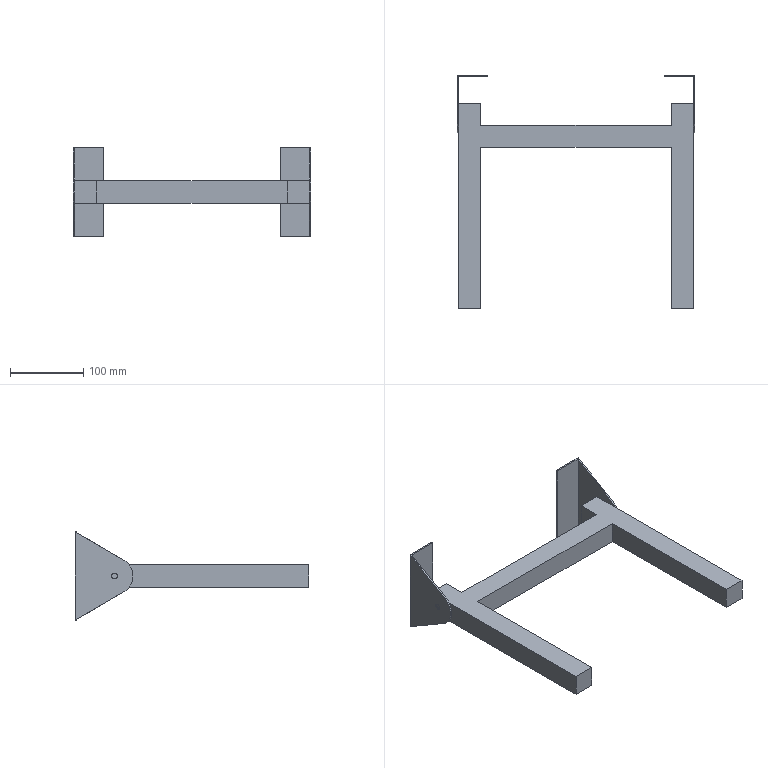Part | NX | 1 solid | 42 faces | box 324 x 318 x 120 mm | volume 780087 mm3 | plane 38 | cylinder 4 | commonest cylinder face diameters 8 x2 50 x2
STEP:
#1=CARTESIAN_POINT('',(-160.,140.,-15.));
#2=VERTEX_POINT('',#1);
#3=CARTESIAN_POINT('',(-160.,104.51,-15.));
#4=VERTEX_POINT('',#3);
#5=CARTESIAN_POINT('',(-160.,140.,-15.));
#6=DIRECTION('',(0.,-1.,0.));
#7=VECTOR('',#6,1.);
#8=LINE('',#5,#7);
#9=EDGE_CURVE('',#2,#4,#8,.T.);
#10=ORIENTED_EDGE('',*,*,#9,.F.);
#11=CARTESIAN_POINT('',(-130.,140.,-15.));
#12=VERTEX_POINT('',#11);
#13=CARTESIAN_POINT('',(-130.,140.,-15.));
#14=DIRECTION('',(-1.,0.,0.));
#15=VECTOR('',#14,1.);
#16=LINE('',#13,#15);
#17=EDGE_CURVE('',#12,#2,#16,.T.);
#18=ORIENTED_EDGE('',*,*,#17,.F.);
#19=CARTESIAN_POINT('',(-130.,110.,-15.));
#20=VERTEX_POINT('',#19);
#21=CARTESIAN_POINT('',(-130.,110.,-15.));
#22=DIRECTION('',(0.,1.,0.));
#23=VECTOR('',#22,1.);
#24=LINE('',#21,#23);
#25=EDGE_CURVE('',#20,#12,#24,.T.);
#26=ORIENTED_EDGE('',*,*,#25,.F.);
#27=CARTESIAN_POINT('',(130.,110.,-15.));
#28=VERTEX_POINT('',#27);
#29=CARTESIAN_POINT('',(130.,110.,-15.));
#30=DIRECTION('',(-1.,0.,0.));
#31=VECTOR('',#30,1.);
#32=LINE('',#29,#31);
#33=EDGE_CURVE('',#28,#20,#32,.T.);
#34=ORIENTED_EDGE('',*,*,#33,.F.);
#35=CARTESIAN_POINT('',(130.,140.,-15.));
#36=VERTEX_POINT('',#35);
#37=CARTESIAN_POINT('',(130.,140.,-15.));
#38=DIRECTION('',(0.,-1.,0.));
#39=VECTOR('',#38,1.);
#40=LINE('',#37,#39);
#41=EDGE_CURVE('',#36,#28,#40,.T.);
#42=ORIENTED_EDGE('',*,*,#41,.F.);
#43=CARTESIAN_POINT('',(160.,140.,-15.));
#44=VERTEX_POINT('',#43);
#45=CARTESIAN_POINT('',(160.,140.,-15.));
#46=DIRECTION('',(-1.,0.,0.));
#47=VECTOR('',#46,1.);
#48=LINE('',#45,#47);
#49=EDGE_CURVE('',#44,#36,#48,.T.);
#50=ORIENTED_EDGE('',*,*,#49,.F.);
#51=CARTESIAN_POINT('',(160.,104.51,-15.));
#52=VERTEX_POINT('',#51);
#53=CARTESIAN_POINT('',(160.,140.,-15.));
#54=DIRECTION('',(0.,-1.,0.));
#55=VECTOR('',#54,1.);
#56=LINE('',#53,#55);
#57=EDGE_CURVE('',#44,#52,#56,.T.);
#58=ORIENTED_EDGE('',*,*,#57,.T.);
#59=CARTESIAN_POINT('',(160.,-140.,-15.));
#60=VERTEX_POINT('',#59);
#61=CARTESIAN_POINT('',(160.,-140.,-15.));
#62=DIRECTION('',(0.,1.,0.));
#63=VECTOR('',#62,1.);
#64=LINE('',#61,#63);
#65=EDGE_CURVE('',#60,#52,#64,.T.);
#66=ORIENTED_EDGE('',*,*,#65,.F.);
#67=CARTESIAN_POINT('',(130.,-140.,-15.));
#68=VERTEX_POINT('',#67);
#69=CARTESIAN_POINT('',(130.,-140.,-15.));
#70=DIRECTION('',(1.,0.,0.));
#71=VECTOR('',#70,1.);
#72=LINE('',#69,#71);
#73=EDGE_CURVE('',#68,#60,#72,.T.);
#74=ORIENTED_EDGE('',*,*,#73,.F.);
#75=CARTESIAN_POINT('',(130.,80.,-15.));
#76=VERTEX_POINT('',#75);
#77=CARTESIAN_POINT('',(130.,80.,-15.));
#78=DIRECTION('',(0.,-1.,0.));
#79=VECTOR('',#78,1.);
#80=LINE('',#77,#79);
#81=EDGE_CURVE('',#76,#68,#80,.T.);
#82=ORIENTED_EDGE('',*,*,#81,.F.);
#83=CARTESIAN_POINT('',(-130.,80.,-15.));
#84=VERTEX_POINT('',#83);
#85=CARTESIAN_POINT('',(-130.,80.,-15.));
#86=DIRECTION('',(1.,0.,0.));
#87=VECTOR('',#86,1.);
#88=LINE('',#85,#87);
#89=EDGE_CURVE('',#84,#76,#88,.T.);
#90=ORIENTED_EDGE('',*,*,#89,.F.);
#91=CARTESIAN_POINT('',(-130.,-140.,-15.));
#92=VERTEX_POINT('',#91);
#93=CARTESIAN_POINT('',(-130.,-140.,-15.));
#94=DIRECTION('',(0.,1.,0.));
#95=VECTOR('',#94,1.);
#96=LINE('',#93,#95);
#97=EDGE_CURVE('',#92,#84,#96,.T.);
#98=ORIENTED_EDGE('',*,*,#97,.F.);
#99=CARTESIAN_POINT('',(-160.,-140.,-15.));
#100=VERTEX_POINT('',#99);
#101=CARTESIAN_POINT('',(-160.,-140.,-15.));
#102=DIRECTION('',(1.,0.,0.));
#103=VECTOR('',#102,1.);
#104=LINE('',#101,#103);
#105=EDGE_CURVE('',#100,#92,#104,.T.);
#106=ORIENTED_EDGE('',*,*,#105,.F.);
#107=CARTESIAN_POINT('',(-160.,104.51,-15.));
#108=DIRECTION('',(0.,-1.,0.));
#109=VECTOR('',#108,1.);
#110=LINE('',#107,#109);
#111=EDGE_CURVE('',#4,#100,#110,.T.);
#112=ORIENTED_EDGE('',*,*,#111,.F.);
#113=EDGE_LOOP('',(#10,#18,#26,#34,#42,#50,#58,#66,#74,#82,#90,#98,#106,#112));
#114=FACE_OUTER_BOUND('',#113,.T.);
#115=CARTESIAN_POINT('',(0.,0.,-15.));
#116=DIRECTION('',(0.,0.,1.));
#117=DIRECTION('',(1.,0.,0.));
#118=AXIS2_PLACEMENT_3D('',#115,#116,#117);
#119=PLANE('',#118);
#120=ADVANCED_FACE('',(#114),#119,.F.);
#121=CARTESIAN_POINT('',(-160.,140.,15.));
#122=VERTEX_POINT('',#121);
#123=CARTESIAN_POINT('',(-160.,104.51,15.));
#124=VERTEX_POINT('',#123);
#125=CARTESIAN_POINT('',(-160.,140.,15.));
#126=DIRECTION('',(0.,-1.,0.));
#127=VECTOR('',#126,1.);
#128=LINE('',#125,#127);
#129=EDGE_CURVE('',#122,#124,#128,.T.);
#130=ORIENTED_EDGE('',*,*,#129,.T.);
#131=CARTESIAN_POINT('',(-160.,-140.,15.));
#132=VERTEX_POINT('',#131);
#133=CARTESIAN_POINT('',(-160.,104.51,15.));
#134=DIRECTION('',(0.,-1.,0.));
#135=VECTOR('',#134,1.);
#136=LINE('',#133,#135);
#137=EDGE_CURVE('',#124,#132,#136,.T.);
#138=ORIENTED_EDGE('',*,*,#137,.T.);
#139=CARTESIAN_POINT('',(-130.,-140.,15.));
#140=VERTEX_POINT('',#139);
#141=CARTESIAN_POINT('',(-160.,-140.,15.));
#142=DIRECTION('',(1.,0.,0.));
#143=VECTOR('',#142,1.);
#144=LINE('',#141,#143);
#145=EDGE_CURVE('',#132,#140,#144,.T.);
#146=ORIENTED_EDGE('',*,*,#145,.T.);
#147=CARTESIAN_POINT('',(-130.,80.,15.));
#148=VERTEX_POINT('',#147);
#149=CARTESIAN_POINT('',(-130.,-140.,15.));
#150=DIRECTION('',(0.,1.,0.));
#151=VECTOR('',#150,1.);
#152=LINE('',#149,#151);
#153=EDGE_CURVE('',#140,#148,#152,.T.);
#154=ORIENTED_EDGE('',*,*,#153,.T.);
#155=CARTESIAN_POINT('',(130.,80.,15.));
#156=VERTEX_POINT('',#155);
#157=CARTESIAN_POINT('',(-130.,80.,15.));
#158=DIRECTION('',(1.,0.,0.));
#159=VECTOR('',#158,1.);
#160=LINE('',#157,#159);
#161=EDGE_CURVE('',#148,#156,#160,.T.);
#162=ORIENTED_EDGE('',*,*,#161,.T.);
#163=CARTESIAN_POINT('',(130.,-140.,15.));
#164=VERTEX_POINT('',#163);
#165=CARTESIAN_POINT('',(130.,80.,15.));
#166=DIRECTION('',(0.,-1.,0.));
#167=VECTOR('',#166,1.);
#168=LINE('',#165,#167);
#169=EDGE_CURVE('',#156,#164,#168,.T.);
#170=ORIENTED_EDGE('',*,*,#169,.T.);
#171=CARTESIAN_POINT('',(160.,-140.,15.));
#172=VERTEX_POINT('',#171);
#173=CARTESIAN_POINT('',(130.,-140.,15.));
#174=DIRECTION('',(1.,0.,0.));
#175=VECTOR('',#174,1.);
#176=LINE('',#173,#175);
#177=EDGE_CURVE('',#164,#172,#176,.T.);
#178=ORIENTED_EDGE('',*,*,#177,.T.);
#179=CARTESIAN_POINT('',(160.,104.51,15.));
#180=VERTEX_POINT('',#179);
#181=CARTESIAN_POINT('',(160.,-140.,15.));
#182=DIRECTION('',(0.,1.,0.));
#183=VECTOR('',#182,1.);
#184=LINE('',#181,#183);
#185=EDGE_CURVE('',#172,#180,#184,.T.);
#186=ORIENTED_EDGE('',*,*,#185,.T.);
#187=CARTESIAN_POINT('',(160.,140.,15.));
#188=VERTEX_POINT('',#187);
#189=CARTESIAN_POINT('',(160.,140.,15.));
#190=DIRECTION('',(0.,-1.,0.));
#191=VECTOR('',#190,1.);
#192=LINE('',#189,#191);
#193=EDGE_CURVE('',#188,#180,#192,.T.);
#194=ORIENTED_EDGE('',*,*,#193,.F.);
#195=CARTESIAN_POINT('',(130.,140.,15.));
#196=VERTEX_POINT('',#195);
#197=CARTESIAN_POINT('',(160.,140.,15.));
#198=DIRECTION('',(-1.,0.,0.));
#199=VECTOR('',#198,1.);
#200=LINE('',#197,#199);
#201=EDGE_CURVE('',#188,#196,#200,.T.);
#202=ORIENTED_EDGE('',*,*,#201,.T.);
#203=CARTESIAN_POINT('',(130.,110.,15.));
#204=VERTEX_POINT('',#203);
#205=CARTESIAN_POINT('',(130.,140.,15.));
#206=DIRECTION('',(0.,-1.,0.));
#207=VECTOR('',#206,1.);
#208=LINE('',#205,#207);
#209=EDGE_CURVE('',#196,#204,#208,.T.);
#210=ORIENTED_EDGE('',*,*,#209,.T.);
#211=CARTESIAN_POINT('',(-130.,110.,15.));
#212=VERTEX_POINT('',#211);
#213=CARTESIAN_POINT('',(130.,110.,15.));
#214=DIRECTION('',(-1.,0.,0.));
#215=VECTOR('',#214,1.);
#216=LINE('',#213,#215);
#217=EDGE_CURVE('',#204,#212,#216,.T.);
#218=ORIENTED_EDGE('',*,*,#217,.T.);
#219=CARTESIAN_POINT('',(-130.,140.,15.));
#220=VERTEX_POINT('',#219);
#221=CARTESIAN_POINT('',(-130.,110.,15.));
#222=DIRECTION('',(0.,1.,0.));
#223=VECTOR('',#222,1.);
#224=LINE('',#221,#223);
#225=EDGE_CURVE('',#212,#220,#224,.T.);
#226=ORIENTED_EDGE('',*,*,#225,.T.);
#227=CARTESIAN_POINT('',(-130.,140.,15.));
#228=DIRECTION('',(-1.,0.,0.));
#229=VECTOR('',#228,1.);
#230=LINE('',#227,#229);
#231=EDGE_CURVE('',#220,#122,#230,.T.);
#232=ORIENTED_EDGE('',*,*,#231,.T.);
#233=EDGE_LOOP('',(#130,#138,#146,#154,#162,#170,#178,#186,#194,#202,#210,#218,#226,#232));
#234=FACE_OUTER_BOUND('',#233,.T.);
#235=CARTESIAN_POINT('',(0.,0.,15.));
#236=DIRECTION('',(0.,0.,1.));
#237=DIRECTION('',(1.,0.,0.));
#238=AXIS2_PLACEMENT_3D('',#235,#236,#237);
#239=PLANE('',#238);
#240=ADVANCED_FACE('',(#234),#239,.T.);
#241=CARTESIAN_POINT('',(130.,80.,-15.));
#242=DIRECTION('',(0.,0.,1.));
#243=VECTOR('',#242,1.);
#244=LINE('',#241,#243);
#245=EDGE_CURVE('',#76,#156,#244,.T.);
#246=ORIENTED_EDGE('',*,*,#245,.F.);
#247=ORIENTED_EDGE('',*,*,#81,.T.);
#248=CARTESIAN_POINT('',(130.,-140.,-15.));
#249=DIRECTION('',(0.,0.,1.));
#250=VECTOR('',#249,1.);
#251=LINE('',#248,#250);
#252=EDGE_CURVE('',#68,#164,#251,.T.);
#253=ORIENTED_EDGE('',*,*,#252,.T.);
#254=ORIENTED_EDGE('',*,*,#169,.F.);
#255=EDGE_LOOP('',(#246,#247,#253,#254));
#256=FACE_OUTER_BOUND('',#255,.T.);
#257=CARTESIAN_POINT('',(130.,140.,-15.));
#258=DIRECTION('',(-1.,0.,0.));
#259=DIRECTION('',(0.,0.,1.));
#260=AXIS2_PLACEMENT_3D('',#257,#258,#259);
#261=PLANE('',#260);
#262=ADVANCED_FACE('',(#256),#261,.T.);
#263=CARTESIAN_POINT('',(130.,110.,-15.));
#264=DIRECTION('',(0.,0.,1.));
#265=VECTOR('',#264,1.);
#266=LINE('',#263,#265);
#267=EDGE_CURVE('',#28,#204,#266,.T.);
#268=ORIENTED_EDGE('',*,*,#267,.T.);
#269=ORIENTED_EDGE('',*,*,#209,.F.);
#270=CARTESIAN_POINT('',(130.,140.,-15.));
#271=DIRECTION('',(0.,0.,1.));
#272=VECTOR('',#271,1.);
#273=LINE('',#270,#272);
#274=EDGE_CURVE('',#36,#196,#273,.T.);
#275=ORIENTED_EDGE('',*,*,#274,.F.);
#276=ORIENTED_EDGE('',*,*,#41,.T.);
#277=EDGE_LOOP('',(#268,#269,#275,#276));
#278=FACE_OUTER_BOUND('',#277,.T.);
#279=CARTESIAN_POINT('',(130.,140.,-15.));
#280=DIRECTION('',(-1.,0.,0.));
#281=DIRECTION('',(0.,0.,1.));
#282=AXIS2_PLACEMENT_3D('',#279,#280,#281);
#283=PLANE('',#282);
#284=ADVANCED_FACE('',(#278),#283,.T.);
#285=ORIENTED_EDGE('',*,*,#73,.T.);
#286=CARTESIAN_POINT('',(160.,-140.,-15.));
#287=DIRECTION('',(0.,0.,1.));
#288=VECTOR('',#287,1.);
#289=LINE('',#286,#288);
#290=EDGE_CURVE('',#60,#172,#289,.T.);
#291=ORIENTED_EDGE('',*,*,#290,.T.);
#292=ORIENTED_EDGE('',*,*,#177,.F.);
#293=ORIENTED_EDGE('',*,*,#252,.F.);
#294=EDGE_LOOP('',(#285,#291,#292,#293));
#295=FACE_OUTER_BOUND('',#294,.T.);
#296=CARTESIAN_POINT('',(130.,-140.,-15.));
#297=DIRECTION('',(0.,-1.,0.));
#298=DIRECTION('',(0.,0.,-1.));
#299=AXIS2_PLACEMENT_3D('',#296,#297,#298);
#300=PLANE('',#299);
#301=ADVANCED_FACE('',(#295),#300,.T.);
#302=ORIENTED_EDGE('',*,*,#65,.T.);
#303=CARTESIAN_POINT('',(160.,124.51,0.));
#304=DIRECTION('',(1.,0.,0.));
#305=DIRECTION('',(0.,-0.8,0.6));
#306=AXIS2_PLACEMENT_3D('',#303,#304,#305);
#307=CIRCLE('',#306,25.);
#308=EDGE_CURVE('',#180,#52,#307,.T.);
#309=ORIENTED_EDGE('',*,*,#308,.F.);
#310=ORIENTED_EDGE('',*,*,#185,.F.);
#311=ORIENTED_EDGE('',*,*,#290,.F.);
#312=EDGE_LOOP('',(#302,#309,#310,#311));
#313=FACE_OUTER_BOUND('',#312,.T.);
#314=CARTESIAN_POINT('',(160.,-140.,-15.));
#315=DIRECTION('',(1.,0.,0.));
#316=DIRECTION('',(0.,0.,-1.));
#317=AXIS2_PLACEMENT_3D('',#314,#315,#316);
#318=PLANE('',#317);
#319=ADVANCED_FACE('',(#313),#318,.T.);
#320=CARTESIAN_POINT('',(160.,120.51,0.));
#321=VERTEX_POINT('',#320);
#322=CARTESIAN_POINT('',(160.,124.51,0.));
#323=DIRECTION('',(1.,0.,0.));
#324=DIRECTION('',(0.,1.,0.));
#325=AXIS2_PLACEMENT_3D('',#322,#323,#324);
#326=CIRCLE('',#325,4.);
#327=EDGE_CURVE('',#321,#321,#326,.T.);
#328=ORIENTED_EDGE('',*,*,#327,.T.);
#329=EDGE_LOOP('',(#328));
#330=FACE_OUTER_BOUND('',#329,.T.);
#331=CARTESIAN_POINT('',(160.,-140.,-15.));
#332=DIRECTION('',(1.,0.,0.));
#333=DIRECTION('',(0.,0.,-1.));
#334=AXIS2_PLACEMENT_3D('',#331,#332,#333);
#335=PLANE('',#334);
#336=ADVANCED_FACE('',(#330),#335,.T.);
#337=ORIENTED_EDGE('',*,*,#49,.T.);
#338=ORIENTED_EDGE('',*,*,#274,.T.);
#339=ORIENTED_EDGE('',*,*,#201,.F.);
#340=CARTESIAN_POINT('',(160.,140.,-15.));
#341=DIRECTION('',(0.,0.,1.));
#342=VECTOR('',#341,1.);
#343=LINE('',#340,#342);
#344=EDGE_CURVE('',#44,#188,#343,.T.);
#345=ORIENTED_EDGE('',*,*,#344,.F.);
#346=EDGE_LOOP('',(#337,#338,#339,#345));
#347=FACE_OUTER_BOUND('',#346,.T.);
#348=CARTESIAN_POINT('',(160.,140.,-15.));
#349=DIRECTION('',(0.,1.,0.));
#350=DIRECTION('',(0.,0.,1.));
#351=AXIS2_PLACEMENT_3D('',#348,#349,#350);
#352=PLANE('',#351);
#353=ADVANCED_FACE('',(#347),#352,.T.);
#354=CARTESIAN_POINT('',(-160.,140.,-15.));
#355=DIRECTION('',(0.,0.,1.));
#356=VECTOR('',#355,1.);
#357=LINE('',#354,#356);
#358=EDGE_CURVE('',#2,#122,#357,.T.);
#359=ORIENTED_EDGE('',*,*,#358,.T.);
#360=ORIENTED_EDGE('',*,*,#231,.F.);
#361=CARTESIAN_POINT('',(-130.,140.,-15.));
#362=DIRECTION('',(0.,0.,1.));
#363=VECTOR('',#362,1.);
#364=LINE('',#361,#363);
#365=EDGE_CURVE('',#12,#220,#364,.T.);
#366=ORIENTED_EDGE('',*,*,#365,.F.);
#367=ORIENTED_EDGE('',*,*,#17,.T.);
#368=EDGE_LOOP('',(#359,#360,#366,#367));
#369=FACE_OUTER_BOUND('',#368,.T.);
#370=CARTESIAN_POINT('',(-130.,140.,-15.));
#371=DIRECTION('',(0.,1.,0.));
#372=DIRECTION('',(0.,0.,1.));
#373=AXIS2_PLACEMENT_3D('',#370,#371,#372);
#374=PLANE('',#373);
#375=ADVANCED_FACE('',(#369),#374,.T.);
#376=CARTESIAN_POINT('',(-160.,128.51,0.));
#377=VERTEX_POINT('',#376);
#378=CARTESIAN_POINT('',(-160.,124.51,0.));
#379=DIRECTION('',(1.,0.,0.));
#380=DIRECTION('',(0.,1.,0.));
#381=AXIS2_PLACEMENT_3D('',#378,#379,#380);
#382=CIRCLE('',#381,4.);
#383=EDGE_CURVE('',#377,#377,#382,.T.);
#384=ORIENTED_EDGE('',*,*,#383,.F.);
#385=EDGE_LOOP('',(#384));
#386=FACE_OUTER_BOUND('',#385,.T.);
#387=CARTESIAN_POINT('',(-160.,140.,-15.));
#388=DIRECTION('',(-1.,0.,0.));
#389=DIRECTION('',(0.,0.,1.));
#390=AXIS2_PLACEMENT_3D('',#387,#388,#389);
#391=PLANE('',#390);
#392=ADVANCED_FACE('',(#386),#391,.T.);
#393=CARTESIAN_POINT('',(-160.,124.51,0.));
#394=DIRECTION('',(1.,0.,0.));
#395=DIRECTION('',(0.,-0.8,0.6));
#396=AXIS2_PLACEMENT_3D('',#393,#394,#395);
#397=CIRCLE('',#396,25.);
#398=EDGE_CURVE('',#124,#4,#397,.T.);
#399=ORIENTED_EDGE('',*,*,#398,.T.);
#400=ORIENTED_EDGE('',*,*,#111,.T.);
#401=CARTESIAN_POINT('',(-160.,-140.,-15.));
#402=DIRECTION('',(0.,0.,1.));
#403=VECTOR('',#402,1.);
#404=LINE('',#401,#403);
#405=EDGE_CURVE('',#100,#132,#404,.T.);
#406=ORIENTED_EDGE('',*,*,#405,.T.);
#407=ORIENTED_EDGE('',*,*,#137,.F.);
#408=EDGE_LOOP('',(#399,#400,#406,#407));
#409=FACE_OUTER_BOUND('',#408,.T.);
#410=CARTESIAN_POINT('',(-160.,140.,-15.));
#411=DIRECTION('',(-1.,0.,0.));
#412=DIRECTION('',(0.,0.,1.));
#413=AXIS2_PLACEMENT_3D('',#410,#411,#412);
#414=PLANE('',#413);
#415=ADVANCED_FACE('',(#409),#414,.T.);
#416=ORIENTED_EDGE('',*,*,#105,.T.);
#417=CARTESIAN_POINT('',(-130.,-140.,-15.));
#418=DIRECTION('',(0.,0.,1.));
#419=VECTOR('',#418,1.);
#420=LINE('',#417,#419);
#421=EDGE_CURVE('',#92,#140,#420,.T.);
#422=ORIENTED_EDGE('',*,*,#421,.T.);
#423=ORIENTED_EDGE('',*,*,#145,.F.);
#424=ORIENTED_EDGE('',*,*,#405,.F.);
#425=EDGE_LOOP('',(#416,#422,#423,#424));
#426=FACE_OUTER_BOUND('',#425,.T.);
#427=CARTESIAN_POINT('',(-160.,-140.,-15.));
#428=DIRECTION('',(0.,-1.,0.));
#429=DIRECTION('',(0.,0.,-1.));
#430=AXIS2_PLACEMENT_3D('',#427,#428,#429);
#431=PLANE('',#430);
#432=ADVANCED_FACE('',(#426),#431,.T.);
#433=CARTESIAN_POINT('',(-130.,80.,-15.));
#434=DIRECTION('',(0.,0.,1.));
#435=VECTOR('',#434,1.);
#436=LINE('',#433,#435);
#437=EDGE_CURVE('',#84,#148,#436,.T.);
#438=ORIENTED_EDGE('',*,*,#437,.T.);
#439=ORIENTED_EDGE('',*,*,#153,.F.);
#440=ORIENTED_EDGE('',*,*,#421,.F.);
#441=ORIENTED_EDGE('',*,*,#97,.T.);
#442=EDGE_LOOP('',(#438,#439,#440,#441));
#443=FACE_OUTER_BOUND('',#442,.T.);
#444=CARTESIAN_POINT('',(-130.,-140.,-15.));
#445=DIRECTION('',(1.,0.,0.));
#446=DIRECTION('',(0.,0.,-1.));
#447=AXIS2_PLACEMENT_3D('',#444,#445,#446);
#448=PLANE('',#447);
#449=ADVANCED_FACE('',(#443),#448,.T.);
#450=CARTESIAN_POINT('',(-130.,110.,-15.));
#451=DIRECTION('',(0.,0.,1.));
#452=VECTOR('',#451,1.);
#453=LINE('',#450,#452);
#454=EDGE_CURVE('',#20,#212,#453,.T.);
#455=ORIENTED_EDGE('',*,*,#454,.F.);
#456=ORIENTED_EDGE('',*,*,#25,.T.);
#457=ORIENTED_EDGE('',*,*,#365,.T.);
#458=ORIENTED_EDGE('',*,*,#225,.F.);
#459=EDGE_LOOP('',(#455,#456,#457,#458));
#460=FACE_OUTER_BOUND('',#459,.T.);
#461=CARTESIAN_POINT('',(-130.,-140.,-15.));
#462=DIRECTION('',(1.,0.,0.));
#463=DIRECTION('',(0.,0.,-1.));
#464=AXIS2_PLACEMENT_3D('',#461,#462,#463);
#465=PLANE('',#464);
#466=ADVANCED_FACE('',(#460),#465,.T.);
#467=ORIENTED_EDGE('',*,*,#245,.T.);
#468=ORIENTED_EDGE('',*,*,#161,.F.);
#469=ORIENTED_EDGE('',*,*,#437,.F.);
#470=ORIENTED_EDGE('',*,*,#89,.T.);
#471=EDGE_LOOP('',(#467,#468,#469,#470));
#472=FACE_OUTER_BOUND('',#471,.T.);
#473=CARTESIAN_POINT('',(-130.,80.,15.));
#474=DIRECTION('',(0.,-1.,0.));
#475=DIRECTION('',(0.,0.,-1.));
#476=AXIS2_PLACEMENT_3D('',#473,#474,#475);
#477=PLANE('',#476);
#478=ADVANCED_FACE('',(#472),#477,.T.);
#479=ORIENTED_EDGE('',*,*,#267,.F.);
#480=ORIENTED_EDGE('',*,*,#33,.T.);
#481=ORIENTED_EDGE('',*,*,#454,.T.);
#482=ORIENTED_EDGE('',*,*,#217,.F.);
#483=EDGE_LOOP('',(#479,#480,#481,#482));
#484=FACE_OUTER_BOUND('',#483,.T.);
#485=CARTESIAN_POINT('',(130.,110.,15.));
#486=DIRECTION('',(0.,1.,0.));
#487=DIRECTION('',(0.,0.,1.));
#488=AXIS2_PLACEMENT_3D('',#485,#486,#487);
#489=PLANE('',#488);
#490=ADVANCED_FACE('',(#484),#489,.T.);
#491=CARTESIAN_POINT('',(160.,176.,58.838));
#492=VERTEX_POINT('',#491);
#493=CARTESIAN_POINT('',(160.,176.,-58.838));
#494=VERTEX_POINT('',#493);
#495=CARTESIAN_POINT('',(160.,176.,58.838));
#496=DIRECTION('',(0.,0.,-1.));
#497=VECTOR('',#496,1.);
#498=LINE('',#495,#497);
#499=EDGE_CURVE('',#492,#494,#498,.T.);
#500=ORIENTED_EDGE('',*,*,#499,.T.);
#501=CARTESIAN_POINT('',(160.,111.949,-21.615));
#502=VERTEX_POINT('',#501);
#503=CARTESIAN_POINT('',(160.,176.,-58.838));
#504=DIRECTION('',(0.,-0.8646,0.5025));
#505=VECTOR('',#504,1.);
#506=LINE('',#503,#505);
#507=EDGE_CURVE('',#494,#502,#506,.T.);
#508=ORIENTED_EDGE('',*,*,#507,.T.);
#509=CARTESIAN_POINT('',(160.,124.51,0.));
#510=DIRECTION('',(-1.,0.,0.));
#511=DIRECTION('',(0.,-0.5025,-0.8646));
#512=AXIS2_PLACEMENT_3D('',#509,#510,#511);
#513=CIRCLE('',#512,25.);
#514=EDGE_CURVE('',#502,#52,#513,.T.);
#515=ORIENTED_EDGE('',*,*,#514,.T.);
#516=ORIENTED_EDGE('',*,*,#57,.F.);
#517=ORIENTED_EDGE('',*,*,#344,.T.);
#518=ORIENTED_EDGE('',*,*,#193,.T.);
#519=CARTESIAN_POINT('',(160.,111.949,21.615));
#520=VERTEX_POINT('',#519);
#521=CARTESIAN_POINT('',(160.,124.51,0.));
#522=DIRECTION('',(-1.,0.,0.));
#523=DIRECTION('',(0.,-0.8,0.6));
#524=AXIS2_PLACEMENT_3D('',#521,#522,#523);
#525=CIRCLE('',#524,25.);
#526=EDGE_CURVE('',#180,#520,#525,.T.);
#527=ORIENTED_EDGE('',*,*,#526,.T.);
#528=CARTESIAN_POINT('',(160.,111.949,21.615));
#529=DIRECTION('',(0.,0.8646,0.5025));
#530=VECTOR('',#529,1.);
#531=LINE('',#528,#530);
#532=EDGE_CURVE('',#520,#492,#531,.T.);
#533=ORIENTED_EDGE('',*,*,#532,.T.);
#534=EDGE_LOOP('',(#500,#508,#515,#516,#517,#518,#527,#533));
#535=FACE_OUTER_BOUND('',#534,.T.);
#536=CARTESIAN_POINT('',(160.,0.,-15.));
#537=DIRECTION('',(1.,0.,0.));
#538=DIRECTION('',(0.,0.,-1.));
#539=AXIS2_PLACEMENT_3D('',#536,#537,#538);
#540=PLANE('',#539);
#541=ADVANCED_FACE('',(#535),#540,.F.);
#542=CARTESIAN_POINT('',(162.,178.,-60.));
#543=VERTEX_POINT('',#542);
#544=CARTESIAN_POINT('',(162.,111.949,-21.615));
#545=VERTEX_POINT('',#544);
#546=CARTESIAN_POINT('',(162.,178.,-60.));
#547=DIRECTION('',(0.,-0.8646,0.5025));
#548=VECTOR('',#547,1.);
#549=LINE('',#546,#548);
#550=EDGE_CURVE('',#543,#545,#549,.T.);
#551=ORIENTED_EDGE('',*,*,#550,.F.);
#552=CARTESIAN_POINT('',(162.,178.,60.));
#553=VERTEX_POINT('',#552);
#554=CARTESIAN_POINT('',(162.,178.,60.));
#555=DIRECTION('',(0.,0.,-1.));
#556=VECTOR('',#555,1.);
#557=LINE('',#554,#556);
#558=EDGE_CURVE('',#553,#543,#557,.T.);
#559=ORIENTED_EDGE('',*,*,#558,.F.);
#560=CARTESIAN_POINT('',(162.,111.949,21.615));
#561=VERTEX_POINT('',#560);
#562=CARTESIAN_POINT('',(162.,111.949,21.615));
#563=DIRECTION('',(0.,0.8646,0.5025));
#564=VECTOR('',#563,1.);
#565=LINE('',#562,#564);
#566=EDGE_CURVE('',#561,#553,#565,.T.);
#567=ORIENTED_EDGE('',*,*,#566,.F.);
#568=CARTESIAN_POINT('',(162.,124.51,0.));
#569=DIRECTION('',(-1.,0.,0.));
#570=DIRECTION('',(0.,-0.5025,-0.8646));
#571=AXIS2_PLACEMENT_3D('',#568,#569,#570);
#572=CIRCLE('',#571,25.);
#573=EDGE_CURVE('',#545,#561,#572,.T.);
#574=ORIENTED_EDGE('',*,*,#573,.F.);
#575=EDGE_LOOP('',(#551,#559,#567,#574));
#576=FACE_BOUND('',#575,.T.);
#577=CARTESIAN_POINT('',(162.,120.51,0.));
#578=VERTEX_POINT('',#577);
#579=CARTESIAN_POINT('',(162.,124.51,0.));
#580=DIRECTION('',(1.,0.,0.));
#581=DIRECTION('',(0.,1.,0.));
#582=AXIS2_PLACEMENT_3D('',#579,#580,#581);
#583=CIRCLE('',#582,4.);
#584=EDGE_CURVE('',#578,#578,#583,.T.);
#585=ORIENTED_EDGE('',*,*,#584,.F.);
#586=EDGE_LOOP('',(#585));
#587=FACE_BOUND('',#586,.T.);
#588=CARTESIAN_POINT('',(162.,0.,-15.));
#589=DIRECTION('',(1.,0.,0.));
#590=DIRECTION('',(0.,0.,-1.));
#591=AXIS2_PLACEMENT_3D('',#588,#589,#590);
#592=PLANE('',#591);
#593=ADVANCED_FACE('',(#576,#587),#592,.T.);
#594=ORIENTED_EDGE('',*,*,#327,.F.);
#595=EDGE_LOOP('',(#594));
#596=FACE_BOUND('',#595,.T.);
#597=ORIENTED_EDGE('',*,*,#584,.T.);
#598=EDGE_LOOP('',(#597));
#599=FACE_BOUND('',#598,.T.);
#600=CARTESIAN_POINT('',(160.,124.51,0.));
#601=DIRECTION('',(1.,0.,0.));
#602=DIRECTION('',(0.,-1.,0.));
#603=AXIS2_PLACEMENT_3D('',#600,#601,#602);
#604=CYLINDRICAL_SURFACE('',#603,4.);
#605=ADVANCED_FACE('',(#596,#599),#604,.F.);
#606=CARTESIAN_POINT('',(160.,178.,-60.));
#607=VERTEX_POINT('',#606);
#608=CARTESIAN_POINT('',(160.,178.,-60.));
#609=DIRECTION('',(0.,-0.8646,0.5025));
#610=VECTOR('',#609,1.);
#611=LINE('',#608,#610);
#612=EDGE_CURVE('',#607,#494,#611,.T.);
#613=ORIENTED_EDGE('',*,*,#612,.F.);
#614=CARTESIAN_POINT('',(162.,178.,-60.));
#615=DIRECTION('',(-1.,0.,0.));
#616=VECTOR('',#615,1.);
#617=LINE('',#614,#616);
#618=EDGE_CURVE('',#543,#607,#617,.T.);
#619=ORIENTED_EDGE('',*,*,#618,.F.);
#620=ORIENTED_EDGE('',*,*,#550,.T.);
#621=CARTESIAN_POINT('',(162.,111.949,-21.615));
#622=DIRECTION('',(-1.,0.,0.));
#623=VECTOR('',#622,1.);
#624=LINE('',#621,#623);
#625=EDGE_CURVE('',#545,#502,#624,.T.);
#626=ORIENTED_EDGE('',*,*,#625,.T.);
#627=ORIENTED_EDGE('',*,*,#507,.F.);
#628=EDGE_LOOP('',(#613,#619,#620,#626,#627));
#629=FACE_OUTER_BOUND('',#628,.T.);
#630=CARTESIAN_POINT('',(160.,111.949,-21.615));
#631=DIRECTION('',(0.,-0.5025,-0.8646));
#632=DIRECTION('',(-1.,0.,0.));
#633=AXIS2_PLACEMENT_3D('',#630,#631,#632);
#634=PLANE('',#633);
#635=ADVANCED_FACE('',(#629),#634,.T.);
#636=CARTESIAN_POINT('',(160.,178.,60.));
#637=VERTEX_POINT('',#636);
#638=CARTESIAN_POINT('',(162.,178.,60.));
#639=DIRECTION('',(-1.,0.,0.));
#640=VECTOR('',#639,1.);
#641=LINE('',#638,#640);
#642=EDGE_CURVE('',#553,#637,#641,.T.);
#643=ORIENTED_EDGE('',*,*,#642,.F.);
#644=ORIENTED_EDGE('',*,*,#558,.T.);
#645=ORIENTED_EDGE('',*,*,#618,.T.);
#646=CARTESIAN_POINT('',(120.,178.,-60.));
#647=VERTEX_POINT('',#646);
#648=CARTESIAN_POINT('',(160.,178.,-60.));
#649=DIRECTION('',(-1.,0.,0.));
#650=VECTOR('',#649,1.);
#651=LINE('',#648,#650);
#652=EDGE_CURVE('',#607,#647,#651,.T.);
#653=ORIENTED_EDGE('',*,*,#652,.T.);
#654=CARTESIAN_POINT('',(120.,178.,60.));
#655=VERTEX_POINT('',#654);
#656=CARTESIAN_POINT('',(120.,178.,-60.));
#657=DIRECTION('',(0.,0.,1.));
#658=VECTOR('',#657,1.);
#659=LINE('',#656,#658);
#660=EDGE_CURVE('',#647,#655,#659,.T.);
#661=ORIENTED_EDGE('',*,*,#660,.T.);
#662=CARTESIAN_POINT('',(120.,178.,60.));
#663=DIRECTION('',(1.,0.,0.));
#664=VECTOR('',#663,1.);
#665=LINE('',#662,#664);
#666=EDGE_CURVE('',#655,#637,#665,.T.);
#667=ORIENTED_EDGE('',*,*,#666,.T.);
#668=EDGE_LOOP('',(#643,#644,#645,#653,#661,#667));
#669=FACE_OUTER_BOUND('',#668,.T.);
#670=CARTESIAN_POINT('',(160.,178.,-60.));
#671=DIRECTION('',(0.,1.,0.));
#672=DIRECTION('',(0.,0.,1.));
#673=AXIS2_PLACEMENT_3D('',#670,#671,#672);
#674=PLANE('',#673);
#675=ADVANCED_FACE('',(#669),#674,.T.);
#676=CARTESIAN_POINT('',(160.,178.,60.));
#677=DIRECTION('',(0.,-0.8646,-0.5025));
#678=VECTOR('',#677,1.);
#679=LINE('',#676,#678);
#680=EDGE_CURVE('',#637,#492,#679,.T.);
#681=ORIENTED_EDGE('',*,*,#680,.T.);
#682=ORIENTED_EDGE('',*,*,#532,.F.);
#683=CARTESIAN_POINT('',(162.,111.949,21.615));
#684=DIRECTION('',(-1.,0.,0.));
#685=VECTOR('',#684,1.);
#686=LINE('',#683,#685);
#687=EDGE_CURVE('',#561,#520,#686,.T.);
#688=ORIENTED_EDGE('',*,*,#687,.F.);
#689=ORIENTED_EDGE('',*,*,#566,.T.);
#690=ORIENTED_EDGE('',*,*,#642,.T.);
#691=EDGE_LOOP('',(#681,#682,#688,#689,#690));
#692=FACE_OUTER_BOUND('',#691,.T.);
#693=CARTESIAN_POINT('',(160.,178.,60.));
#694=DIRECTION('',(0.,-0.5025,0.8646));
#695=DIRECTION('',(1.,0.,0.));
#696=AXIS2_PLACEMENT_3D('',#693,#694,#695);
#697=PLANE('',#696);
#698=ADVANCED_FACE('',(#692),#697,.T.);
#699=ORIENTED_EDGE('',*,*,#526,.F.);
#700=ORIENTED_EDGE('',*,*,#308,.T.);
#701=ORIENTED_EDGE('',*,*,#514,.F.);
#702=ORIENTED_EDGE('',*,*,#625,.F.);
#703=ORIENTED_EDGE('',*,*,#573,.T.);
#704=ORIENTED_EDGE('',*,*,#687,.T.);
#705=EDGE_LOOP('',(#699,#700,#701,#702,#703,#704));
#706=FACE_OUTER_BOUND('',#705,.T.);
#707=CARTESIAN_POINT('',(160.,124.51,0.));
#708=DIRECTION('',(1.,0.,0.));
#709=DIRECTION('',(0.,-1.,0.));
#710=AXIS2_PLACEMENT_3D('',#707,#708,#709);
#711=CYLINDRICAL_SURFACE('',#710,25.);
#712=ADVANCED_FACE('',(#706),#711,.T.);
#713=ORIENTED_EDGE('',*,*,#499,.F.);
#714=CARTESIAN_POINT('',(160.,176.,60.));
#715=VERTEX_POINT('',#714);
#716=CARTESIAN_POINT('',(160.,176.,60.));
#717=DIRECTION('',(0.,0.,-1.));
#718=VECTOR('',#717,1.);
#719=LINE('',#716,#718);
#720=EDGE_CURVE('',#715,#492,#719,.T.);
#721=ORIENTED_EDGE('',*,*,#720,.F.);
#722=CARTESIAN_POINT('',(120.,176.,60.));
#723=VERTEX_POINT('',#722);
#724=CARTESIAN_POINT('',(120.,176.,60.));
#725=DIRECTION('',(1.,0.,0.));
#726=VECTOR('',#725,1.);
#727=LINE('',#724,#726);
#728=EDGE_CURVE('',#723,#715,#727,.T.);
#729=ORIENTED_EDGE('',*,*,#728,.F.);
#730=CARTESIAN_POINT('',(120.,176.,-60.));
#731=VERTEX_POINT('',#730);
#732=CARTESIAN_POINT('',(120.,176.,-60.));
#733=DIRECTION('',(0.,0.,1.));
#734=VECTOR('',#733,1.);
#735=LINE('',#732,#734);
#736=EDGE_CURVE('',#731,#723,#735,.T.);
#737=ORIENTED_EDGE('',*,*,#736,.F.);
#738=CARTESIAN_POINT('',(160.,176.,-60.));
#739=VERTEX_POINT('',#738);
#740=CARTESIAN_POINT('',(160.,176.,-60.));
#741=DIRECTION('',(-1.,0.,0.));
#742=VECTOR('',#741,1.);
#743=LINE('',#740,#742);
#744=EDGE_CURVE('',#739,#731,#743,.T.);
#745=ORIENTED_EDGE('',*,*,#744,.F.);
#746=CARTESIAN_POINT('',(160.,176.,-58.838));
#747=DIRECTION('',(0.,0.,-1.));
#748=VECTOR('',#747,1.);
#749=LINE('',#746,#748);
#750=EDGE_CURVE('',#494,#739,#749,.T.);
#751=ORIENTED_EDGE('',*,*,#750,.F.);
#752=EDGE_LOOP('',(#713,#721,#729,#737,#745,#751));
#753=FACE_OUTER_BOUND('',#752,.T.);
#754=CARTESIAN_POINT('',(160.,176.,-15.));
#755=DIRECTION('',(0.,1.,0.));
#756=DIRECTION('',(0.,0.,1.));
#757=AXIS2_PLACEMENT_3D('',#754,#755,#756);
#758=PLANE('',#757);
#759=ADVANCED_FACE('',(#753),#758,.F.);
#760=ORIENTED_EDGE('',*,*,#652,.F.);
#761=CARTESIAN_POINT('',(160.,178.,-60.));
#762=DIRECTION('',(0.,-1.,0.));
#763=VECTOR('',#762,1.);
#764=LINE('',#761,#763);
#765=EDGE_CURVE('',#607,#739,#764,.T.);
#766=ORIENTED_EDGE('',*,*,#765,.T.);
#767=ORIENTED_EDGE('',*,*,#744,.T.);
#768=CARTESIAN_POINT('',(120.,178.,-60.));
#769=DIRECTION('',(0.,-1.,0.));
#770=VECTOR('',#769,1.);
#771=LINE('',#768,#770);
#772=EDGE_CURVE('',#647,#731,#771,.T.);
#773=ORIENTED_EDGE('',*,*,#772,.F.);
#774=EDGE_LOOP('',(#760,#766,#767,#773));
#775=FACE_OUTER_BOUND('',#774,.T.);
#776=CARTESIAN_POINT('',(160.,178.,-60.));
#777=DIRECTION('',(0.,0.,-1.));
#778=DIRECTION('',(-1.,0.,0.));
#779=AXIS2_PLACEMENT_3D('',#776,#777,#778);
#780=PLANE('',#779);
#781=ADVANCED_FACE('',(#775),#780,.T.);
#782=ORIENTED_EDGE('',*,*,#660,.F.);
#783=ORIENTED_EDGE('',*,*,#772,.T.);
#784=ORIENTED_EDGE('',*,*,#736,.T.);
#785=CARTESIAN_POINT('',(120.,178.,60.));
#786=DIRECTION('',(0.,-1.,0.));
#787=VECTOR('',#786,1.);
#788=LINE('',#785,#787);
#789=EDGE_CURVE('',#655,#723,#788,.T.);
#790=ORIENTED_EDGE('',*,*,#789,.F.);
#791=EDGE_LOOP('',(#782,#783,#784,#790));
#792=FACE_OUTER_BOUND('',#791,.T.);
#793=CARTESIAN_POINT('',(120.,178.,-60.));
#794=DIRECTION('',(-1.,0.,0.));
#795=DIRECTION('',(0.,0.,1.));
#796=AXIS2_PLACEMENT_3D('',#793,#794,#795);
#797=PLANE('',#796);
#798=ADVANCED_FACE('',(#792),#797,.T.);
#799=ORIENTED_EDGE('',*,*,#666,.F.);
#800=ORIENTED_EDGE('',*,*,#789,.T.);
#801=ORIENTED_EDGE('',*,*,#728,.T.);
#802=CARTESIAN_POINT('',(160.,178.,60.));
#803=DIRECTION('',(0.,-1.,0.));
#804=VECTOR('',#803,1.);
#805=LINE('',#802,#804);
#806=EDGE_CURVE('',#637,#715,#805,.T.);
#807=ORIENTED_EDGE('',*,*,#806,.F.);
#808=EDGE_LOOP('',(#799,#800,#801,#807));
#809=FACE_OUTER_BOUND('',#808,.T.);
#810=CARTESIAN_POINT('',(120.,178.,60.));
#811=DIRECTION('',(0.,0.,1.));
#812=DIRECTION('',(1.,0.,0.));
#813=AXIS2_PLACEMENT_3D('',#810,#811,#812);
#814=PLANE('',#813);
#815=ADVANCED_FACE('',(#809),#814,.T.);
#816=ORIENTED_EDGE('',*,*,#612,.T.);
#817=ORIENTED_EDGE('',*,*,#750,.T.);
#818=ORIENTED_EDGE('',*,*,#765,.F.);
#819=EDGE_LOOP('',(#816,#817,#818));
#820=FACE_OUTER_BOUND('',#819,.T.);
#821=CARTESIAN_POINT('',(160.,178.,60.));
#822=DIRECTION('',(1.,0.,0.));
#823=DIRECTION('',(0.,0.,-1.));
#824=AXIS2_PLACEMENT_3D('',#821,#822,#823);
#825=PLANE('',#824);
#826=ADVANCED_FACE('',(#820),#825,.T.);
#827=ORIENTED_EDGE('',*,*,#680,.F.);
#828=ORIENTED_EDGE('',*,*,#806,.T.);
#829=ORIENTED_EDGE('',*,*,#720,.T.);
#830=EDGE_LOOP('',(#827,#828,#829));
#831=FACE_OUTER_BOUND('',#830,.T.);
#832=CARTESIAN_POINT('',(160.,178.,60.));
#833=DIRECTION('',(1.,0.,0.));
#834=DIRECTION('',(0.,0.,-1.));
#835=AXIS2_PLACEMENT_3D('',#832,#833,#834);
#836=PLANE('',#835);
#837=ADVANCED_FACE('',(#831),#836,.T.);
#838=CARTESIAN_POINT('',(-160.,176.,58.838));
#839=VERTEX_POINT('',#838);
#840=CARTESIAN_POINT('',(-160.,176.,-58.838));
#841=VERTEX_POINT('',#840);
#842=CARTESIAN_POINT('',(-160.,176.,58.838));
#843=DIRECTION('',(0.,0.,-1.));
#844=VECTOR('',#843,1.);
#845=LINE('',#842,#844);
#846=EDGE_CURVE('',#839,#841,#845,.T.);
#847=ORIENTED_EDGE('',*,*,#846,.F.);
#848=CARTESIAN_POINT('',(-160.,111.949,21.615));
#849=VERTEX_POINT('',#848);
#850=CARTESIAN_POINT('',(-160.,176.,58.838));
#851=DIRECTION('',(0.,-0.8646,-0.5025));
#852=VECTOR('',#851,1.);
#853=LINE('',#850,#852);
#854=EDGE_CURVE('',#839,#849,#853,.T.);
#855=ORIENTED_EDGE('',*,*,#854,.T.);
#856=CARTESIAN_POINT('',(-160.,124.51,0.));
#857=DIRECTION('',(1.,0.,0.));
#858=DIRECTION('',(0.,-0.5025,0.8646));
#859=AXIS2_PLACEMENT_3D('',#856,#857,#858);
#860=CIRCLE('',#859,25.);
#861=EDGE_CURVE('',#849,#124,#860,.T.);
#862=ORIENTED_EDGE('',*,*,#861,.T.);
#863=ORIENTED_EDGE('',*,*,#129,.F.);
#864=ORIENTED_EDGE('',*,*,#358,.F.);
#865=ORIENTED_EDGE('',*,*,#9,.T.);
#866=CARTESIAN_POINT('',(-160.,111.949,-21.615));
#867=VERTEX_POINT('',#866);
#868=CARTESIAN_POINT('',(-160.,124.51,0.));
#869=DIRECTION('',(1.,0.,0.));
#870=DIRECTION('',(0.,-0.8,-0.6));
#871=AXIS2_PLACEMENT_3D('',#868,#869,#870);
#872=CIRCLE('',#871,25.);
#873=EDGE_CURVE('',#4,#867,#872,.T.);
#874=ORIENTED_EDGE('',*,*,#873,.T.);
#875=CARTESIAN_POINT('',(-160.,111.949,-21.615));
#876=DIRECTION('',(0.,0.8646,-0.5025));
#877=VECTOR('',#876,1.);
#878=LINE('',#875,#877);
#879=EDGE_CURVE('',#867,#841,#878,.T.);
#880=ORIENTED_EDGE('',*,*,#879,.T.);
#881=EDGE_LOOP('',(#847,#855,#862,#863,#864,#865,#874,#880));
#882=FACE_OUTER_BOUND('',#881,.T.);
#883=CARTESIAN_POINT('',(-160.,0.,-15.));
#884=DIRECTION('',(1.,0.,0.));
#885=DIRECTION('',(0.,0.,-1.));
#886=AXIS2_PLACEMENT_3D('',#883,#884,#885);
#887=PLANE('',#886);
#888=ADVANCED_FACE('',(#882),#887,.T.);
#889=CARTESIAN_POINT('',(-162.,111.949,-21.615));
#890=VERTEX_POINT('',#889);
#891=CARTESIAN_POINT('',(-162.,178.,-60.));
#892=VERTEX_POINT('',#891);
#893=CARTESIAN_POINT('',(-162.,111.949,-21.615));
#894=DIRECTION('',(0.,0.8646,-0.5025));
#895=VECTOR('',#894,1.);
#896=LINE('',#893,#895);
#897=EDGE_CURVE('',#890,#892,#896,.T.);
#898=ORIENTED_EDGE('',*,*,#897,.F.);
#899=CARTESIAN_POINT('',(-162.,111.949,21.615));
#900=VERTEX_POINT('',#899);
#901=CARTESIAN_POINT('',(-162.,124.51,0.));
#902=DIRECTION('',(1.,0.,0.));
#903=DIRECTION('',(0.,-0.5025,0.8646));
#904=AXIS2_PLACEMENT_3D('',#901,#902,#903);
#905=CIRCLE('',#904,25.);
#906=EDGE_CURVE('',#900,#890,#905,.T.);
#907=ORIENTED_EDGE('',*,*,#906,.F.);
#908=CARTESIAN_POINT('',(-162.,178.,60.));
#909=VERTEX_POINT('',#908);
#910=CARTESIAN_POINT('',(-162.,178.,60.));
#911=DIRECTION('',(0.,-0.8646,-0.5025));
#912=VECTOR('',#911,1.);
#913=LINE('',#910,#912);
#914=EDGE_CURVE('',#909,#900,#913,.T.);
#915=ORIENTED_EDGE('',*,*,#914,.F.);
#916=CARTESIAN_POINT('',(-162.,178.,-60.));
#917=DIRECTION('',(0.,0.,1.));
#918=VECTOR('',#917,1.);
#919=LINE('',#916,#918);
#920=EDGE_CURVE('',#892,#909,#919,.T.);
#921=ORIENTED_EDGE('',*,*,#920,.F.);
#922=EDGE_LOOP('',(#898,#907,#915,#921));
#923=FACE_BOUND('',#922,.T.);
#924=CARTESIAN_POINT('',(-162.,128.51,0.));
#925=VERTEX_POINT('',#924);
#926=CARTESIAN_POINT('',(-162.,124.51,0.));
#927=DIRECTION('',(-1.,0.,0.));
#928=DIRECTION('',(0.,-1.,0.));
#929=AXIS2_PLACEMENT_3D('',#926,#927,#928);
#930=CIRCLE('',#929,4.);
#931=EDGE_CURVE('',#925,#925,#930,.T.);
#932=ORIENTED_EDGE('',*,*,#931,.F.);
#933=EDGE_LOOP('',(#932));
#934=FACE_BOUND('',#933,.T.);
#935=CARTESIAN_POINT('',(-162.,0.,-15.));
#936=DIRECTION('',(1.,0.,0.));
#937=DIRECTION('',(0.,0.,-1.));
#938=AXIS2_PLACEMENT_3D('',#935,#936,#937);
#939=PLANE('',#938);
#940=ADVANCED_FACE('',(#923,#934),#939,.F.);
#941=ORIENTED_EDGE('',*,*,#383,.T.);
#942=EDGE_LOOP('',(#941));
#943=FACE_BOUND('',#942,.T.);
#944=ORIENTED_EDGE('',*,*,#931,.T.);
#945=EDGE_LOOP('',(#944));
#946=FACE_BOUND('',#945,.T.);
#947=CARTESIAN_POINT('',(-160.,124.51,0.));
#948=DIRECTION('',(1.,0.,0.));
#949=DIRECTION('',(0.,-1.,0.));
#950=AXIS2_PLACEMENT_3D('',#947,#948,#949);
#951=CYLINDRICAL_SURFACE('',#950,4.);
#952=ADVANCED_FACE('',(#943,#946),#951,.F.);
#953=CARTESIAN_POINT('',(-160.,178.,-60.));
#954=VERTEX_POINT('',#953);
#955=CARTESIAN_POINT('',(-160.,178.,-60.));
#956=DIRECTION('',(0.,-0.8646,0.5025));
#957=VECTOR('',#956,1.);
#958=LINE('',#955,#957);
#959=EDGE_CURVE('',#954,#841,#958,.T.);
#960=ORIENTED_EDGE('',*,*,#959,.T.);
#961=ORIENTED_EDGE('',*,*,#879,.F.);
#962=CARTESIAN_POINT('',(-160.,111.949,-21.615));
#963=DIRECTION('',(-1.,0.,0.));
#964=VECTOR('',#963,1.);
#965=LINE('',#962,#964);
#966=EDGE_CURVE('',#867,#890,#965,.T.);
#967=ORIENTED_EDGE('',*,*,#966,.T.);
#968=ORIENTED_EDGE('',*,*,#897,.T.);
#969=CARTESIAN_POINT('',(-160.,178.,-60.));
#970=DIRECTION('',(-1.,0.,0.));
#971=VECTOR('',#970,1.);
#972=LINE('',#969,#971);
#973=EDGE_CURVE('',#954,#892,#972,.T.);
#974=ORIENTED_EDGE('',*,*,#973,.F.);
#975=EDGE_LOOP('',(#960,#961,#967,#968,#974));
#976=FACE_OUTER_BOUND('',#975,.T.);
#977=CARTESIAN_POINT('',(-160.,111.949,-21.615));
#978=DIRECTION('',(0.,0.5025,0.8646));
#979=DIRECTION('',(1.,0.,0.));
#980=AXIS2_PLACEMENT_3D('',#977,#978,#979);
#981=PLANE('',#980);
#982=ADVANCED_FACE('',(#976),#981,.F.);
#983=ORIENTED_EDGE('',*,*,#973,.T.);
#984=ORIENTED_EDGE('',*,*,#920,.T.);
#985=CARTESIAN_POINT('',(-160.,178.,60.));
#986=VERTEX_POINT('',#985);
#987=CARTESIAN_POINT('',(-160.,178.,60.));
#988=DIRECTION('',(-1.,0.,0.));
#989=VECTOR('',#988,1.);
#990=LINE('',#987,#989);
#991=EDGE_CURVE('',#986,#909,#990,.T.);
#992=ORIENTED_EDGE('',*,*,#991,.F.);
#993=CARTESIAN_POINT('',(-120.,178.,60.));
#994=VERTEX_POINT('',#993);
#995=CARTESIAN_POINT('',(-120.,178.,60.));
#996=DIRECTION('',(-1.,0.,0.));
#997=VECTOR('',#996,1.);
#998=LINE('',#995,#997);
#999=EDGE_CURVE('',#994,#986,#998,.T.);
#1000=ORIENTED_EDGE('',*,*,#999,.F.);
#1001=CARTESIAN_POINT('',(-120.,178.,-60.));
#1002=VERTEX_POINT('',#1001);
#1003=CARTESIAN_POINT('',(-120.,178.,-60.));
#1004=DIRECTION('',(0.,0.,1.));
#1005=VECTOR('',#1004,1.);
#1006=LINE('',#1003,#1005);
#1007=EDGE_CURVE('',#1002,#994,#1006,.T.);
#1008=ORIENTED_EDGE('',*,*,#1007,.F.);
#1009=CARTESIAN_POINT('',(-160.,178.,-60.));
#1010=DIRECTION('',(1.,0.,0.));
#1011=VECTOR('',#1010,1.);
#1012=LINE('',#1009,#1011);
#1013=EDGE_CURVE('',#954,#1002,#1012,.T.);
#1014=ORIENTED_EDGE('',*,*,#1013,.F.);
#1015=EDGE_LOOP('',(#983,#984,#992,#1000,#1008,#1014));
#1016=FACE_OUTER_BOUND('',#1015,.T.);
#1017=CARTESIAN_POINT('',(-160.,178.,-60.));
#1018=DIRECTION('',(0.,-1.,0.));
#1019=DIRECTION('',(0.,0.,-1.));
#1020=AXIS2_PLACEMENT_3D('',#1017,#1018,#1019);
#1021=PLANE('',#1020);
#1022=ADVANCED_FACE('',(#1016),#1021,.F.);
#1023=CARTESIAN_POINT('',(-160.,178.,60.));
#1024=DIRECTION('',(0.,-0.8646,-0.5025));
#1025=VECTOR('',#1024,1.);
#1026=LINE('',#1023,#1025);
#1027=EDGE_CURVE('',#986,#839,#1026,.T.);
#1028=ORIENTED_EDGE('',*,*,#1027,.F.);
#1029=ORIENTED_EDGE('',*,*,#991,.T.);
#1030=ORIENTED_EDGE('',*,*,#914,.T.);
#1031=CARTESIAN_POINT('',(-160.,111.949,21.615));
#1032=DIRECTION('',(-1.,0.,0.));
#1033=VECTOR('',#1032,1.);
#1034=LINE('',#1031,#1033);
#1035=EDGE_CURVE('',#849,#900,#1034,.T.);
#1036=ORIENTED_EDGE('',*,*,#1035,.F.);
#1037=ORIENTED_EDGE('',*,*,#854,.F.);
#1038=EDGE_LOOP('',(#1028,#1029,#1030,#1036,#1037));
#1039=FACE_OUTER_BOUND('',#1038,.T.);
#1040=CARTESIAN_POINT('',(-160.,178.,60.));
#1041=DIRECTION('',(0.,0.5025,-0.8646));
#1042=DIRECTION('',(-1.,0.,0.));
#1043=AXIS2_PLACEMENT_3D('',#1040,#1041,#1042);
#1044=PLANE('',#1043);
#1045=ADVANCED_FACE('',(#1039),#1044,.F.);
#1046=ORIENTED_EDGE('',*,*,#398,.F.);
#1047=ORIENTED_EDGE('',*,*,#861,.F.);
#1048=ORIENTED_EDGE('',*,*,#1035,.T.);
#1049=ORIENTED_EDGE('',*,*,#906,.T.);
#1050=ORIENTED_EDGE('',*,*,#966,.F.);
#1051=ORIENTED_EDGE('',*,*,#873,.F.);
#1052=EDGE_LOOP('',(#1046,#1047,#1048,#1049,#1050,#1051));
#1053=FACE_OUTER_BOUND('',#1052,.T.);
#1054=CARTESIAN_POINT('',(-160.,124.51,0.));
#1055=DIRECTION('',(1.,0.,0.));
#1056=DIRECTION('',(0.,-1.,0.));
#1057=AXIS2_PLACEMENT_3D('',#1054,#1055,#1056);
#1058=CYLINDRICAL_SURFACE('',#1057,25.);
#1059=ADVANCED_FACE('',(#1053),#1058,.T.);
#1060=ORIENTED_EDGE('',*,*,#846,.T.);
#1061=CARTESIAN_POINT('',(-160.,176.,-60.));
#1062=VERTEX_POINT('',#1061);
#1063=CARTESIAN_POINT('',(-160.,176.,-58.838));
#1064=DIRECTION('',(0.,0.,-1.));
#1065=VECTOR('',#1064,1.);
#1066=LINE('',#1063,#1065);
#1067=EDGE_CURVE('',#841,#1062,#1066,.T.);
#1068=ORIENTED_EDGE('',*,*,#1067,.T.);
#1069=CARTESIAN_POINT('',(-120.,176.,-60.));
#1070=VERTEX_POINT('',#1069);
#1071=CARTESIAN_POINT('',(-160.,176.,-60.));
#1072=DIRECTION('',(1.,0.,0.));
#1073=VECTOR('',#1072,1.);
#1074=LINE('',#1071,#1073);
#1075=EDGE_CURVE('',#1062,#1070,#1074,.T.);
#1076=ORIENTED_EDGE('',*,*,#1075,.T.);
#1077=CARTESIAN_POINT('',(-120.,176.,60.));
#1078=VERTEX_POINT('',#1077);
#1079=CARTESIAN_POINT('',(-120.,176.,-60.));
#1080=DIRECTION('',(0.,0.,1.));
#1081=VECTOR('',#1080,1.);
#1082=LINE('',#1079,#1081);
#1083=EDGE_CURVE('',#1070,#1078,#1082,.T.);
#1084=ORIENTED_EDGE('',*,*,#1083,.T.);
#1085=CARTESIAN_POINT('',(-160.,176.,60.));
#1086=VERTEX_POINT('',#1085);
#1087=CARTESIAN_POINT('',(-120.,176.,60.));
#1088=DIRECTION('',(-1.,0.,0.));
#1089=VECTOR('',#1088,1.);
#1090=LINE('',#1087,#1089);
#1091=EDGE_CURVE('',#1078,#1086,#1090,.T.);
#1092=ORIENTED_EDGE('',*,*,#1091,.T.);
#1093=CARTESIAN_POINT('',(-160.,176.,60.));
#1094=DIRECTION('',(0.,0.,-1.));
#1095=VECTOR('',#1094,1.);
#1096=LINE('',#1093,#1095);
#1097=EDGE_CURVE('',#1086,#839,#1096,.T.);
#1098=ORIENTED_EDGE('',*,*,#1097,.T.);
#1099=EDGE_LOOP('',(#1060,#1068,#1076,#1084,#1092,#1098));
#1100=FACE_OUTER_BOUND('',#1099,.T.);
#1101=CARTESIAN_POINT('',(-160.,176.,-15.));
#1102=DIRECTION('',(0.,-1.,0.));
#1103=DIRECTION('',(0.,0.,-1.));
#1104=AXIS2_PLACEMENT_3D('',#1101,#1102,#1103);
#1105=PLANE('',#1104);
#1106=ADVANCED_FACE('',(#1100),#1105,.T.);
#1107=ORIENTED_EDGE('',*,*,#1013,.T.);
#1108=CARTESIAN_POINT('',(-120.,178.,-60.));
#1109=DIRECTION('',(0.,-1.,0.));
#1110=VECTOR('',#1109,1.);
#1111=LINE('',#1108,#1110);
#1112=EDGE_CURVE('',#1002,#1070,#1111,.T.);
#1113=ORIENTED_EDGE('',*,*,#1112,.T.);
#1114=ORIENTED_EDGE('',*,*,#1075,.F.);
#1115=CARTESIAN_POINT('',(-160.,178.,-60.));
#1116=DIRECTION('',(0.,-1.,0.));
#1117=VECTOR('',#1116,1.);
#1118=LINE('',#1115,#1117);
#1119=EDGE_CURVE('',#954,#1062,#1118,.T.);
#1120=ORIENTED_EDGE('',*,*,#1119,.F.);
#1121=EDGE_LOOP('',(#1107,#1113,#1114,#1120));
#1122=FACE_OUTER_BOUND('',#1121,.T.);
#1123=CARTESIAN_POINT('',(-160.,178.,-60.));
#1124=DIRECTION('',(0.,0.,1.));
#1125=DIRECTION('',(1.,0.,0.));
#1126=AXIS2_PLACEMENT_3D('',#1123,#1124,#1125);
#1127=PLANE('',#1126);
#1128=ADVANCED_FACE('',(#1122),#1127,.F.);
#1129=ORIENTED_EDGE('',*,*,#1007,.T.);
#1130=CARTESIAN_POINT('',(-120.,178.,60.));
#1131=DIRECTION('',(0.,-1.,0.));
#1132=VECTOR('',#1131,1.);
#1133=LINE('',#1130,#1132);
#1134=EDGE_CURVE('',#994,#1078,#1133,.T.);
#1135=ORIENTED_EDGE('',*,*,#1134,.T.);
#1136=ORIENTED_EDGE('',*,*,#1083,.F.);
#1137=ORIENTED_EDGE('',*,*,#1112,.F.);
#1138=EDGE_LOOP('',(#1129,#1135,#1136,#1137));
#1139=FACE_OUTER_BOUND('',#1138,.T.);
#1140=CARTESIAN_POINT('',(-120.,178.,-60.));
#1141=DIRECTION('',(-1.,0.,0.));
#1142=DIRECTION('',(0.,0.,1.));
#1143=AXIS2_PLACEMENT_3D('',#1140,#1141,#1142);
#1144=PLANE('',#1143);
#1145=ADVANCED_FACE('',(#1139),#1144,.F.);
#1146=ORIENTED_EDGE('',*,*,#999,.T.);
#1147=CARTESIAN_POINT('',(-160.,178.,60.));
#1148=DIRECTION('',(0.,-1.,0.));
#1149=VECTOR('',#1148,1.);
#1150=LINE('',#1147,#1149);
#1151=EDGE_CURVE('',#986,#1086,#1150,.T.);
#1152=ORIENTED_EDGE('',*,*,#1151,.T.);
#1153=ORIENTED_EDGE('',*,*,#1091,.F.);
#1154=ORIENTED_EDGE('',*,*,#1134,.F.);
#1155=EDGE_LOOP('',(#1146,#1152,#1153,#1154));
#1156=FACE_OUTER_BOUND('',#1155,.T.);
#1157=CARTESIAN_POINT('',(-120.,178.,60.));
#1158=DIRECTION('',(0.,0.,-1.));
#1159=DIRECTION('',(-1.,0.,0.));
#1160=AXIS2_PLACEMENT_3D('',#1157,#1158,#1159);
#1161=PLANE('',#1160);
#1162=ADVANCED_FACE('',(#1156),#1161,.F.);
#1163=ORIENTED_EDGE('',*,*,#959,.F.);
#1164=ORIENTED_EDGE('',*,*,#1119,.T.);
#1165=ORIENTED_EDGE('',*,*,#1067,.F.);
#1166=EDGE_LOOP('',(#1163,#1164,#1165));
#1167=FACE_OUTER_BOUND('',#1166,.T.);
#1168=CARTESIAN_POINT('',(-160.,178.,60.));
#1169=DIRECTION('',(1.,0.,0.));
#1170=DIRECTION('',(0.,0.,-1.));
#1171=AXIS2_PLACEMENT_3D('',#1168,#1169,#1170);
#1172=PLANE('',#1171);
#1173=ADVANCED_FACE('',(#1167),#1172,.F.);
#1174=ORIENTED_EDGE('',*,*,#1027,.T.);
#1175=ORIENTED_EDGE('',*,*,#1097,.F.);
#1176=ORIENTED_EDGE('',*,*,#1151,.F.);
#1177=EDGE_LOOP('',(#1174,#1175,#1176));
#1178=FACE_OUTER_BOUND('',#1177,.T.);
#1179=CARTESIAN_POINT('',(-160.,178.,60.));
#1180=DIRECTION('',(1.,0.,0.));
#1181=DIRECTION('',(0.,0.,-1.));
#1182=AXIS2_PLACEMENT_3D('',#1179,#1180,#1181);
#1183=PLANE('',#1182);
#1184=ADVANCED_FACE('',(#1178),#1183,.F.);
#1185=CLOSED_SHELL('',(#120,#240,#262,#284,#301,#319,#336,#353,#375,#392,#415,#432,#449,#466,#478,#490,#541,#593,#605,#635,#675,#698,#712,#759,#781,#798,#815,#826,#837,#888,#940,#952,#982,#1022,#1045,#1059,#1106,#1128,#1145,#1162,#1173,#1184));
#1186=MANIFOLD_SOLID_BREP('',#1185);
#1187=(LENGTH_UNIT()NAMED_UNIT(*)SI_UNIT(.MILLI.,.METRE.));
#1188=UNCERTAINTY_MEASURE_WITH_UNIT(LENGTH_MEASURE(0.00002),#1187,'','');
#1189=(NAMED_UNIT(*)PLANE_ANGLE_UNIT()SI_UNIT($,.RADIAN.));
#1190=PLANE_ANGLE_MEASURE_WITH_UNIT(PLANE_ANGLE_MEASURE(0.01745),#1189);
#1191=DIMENSIONAL_EXPONENTS(0.,0.,0.,0.,0.,0.,0.);
#1192=(CONVERSION_BASED_UNIT('DEGREE',#1190)NAMED_UNIT(#1191)PLANE_ANGLE_UNIT());
#1193=(NAMED_UNIT(*)SI_UNIT($,.STERADIAN.)SOLID_ANGLE_UNIT());
#1194=(GEOMETRIC_REPRESENTATION_CONTEXT(3)GLOBAL_UNCERTAINTY_ASSIGNED_CONTEXT((#1188))GLOBAL_UNIT_ASSIGNED_CONTEXT((#1187,#1192,#1193))REPRESENTATION_CONTEXT('',''));
#1195=ADVANCED_BREP_SHAPE_REPRESENTATION('',(#1186),#1194);